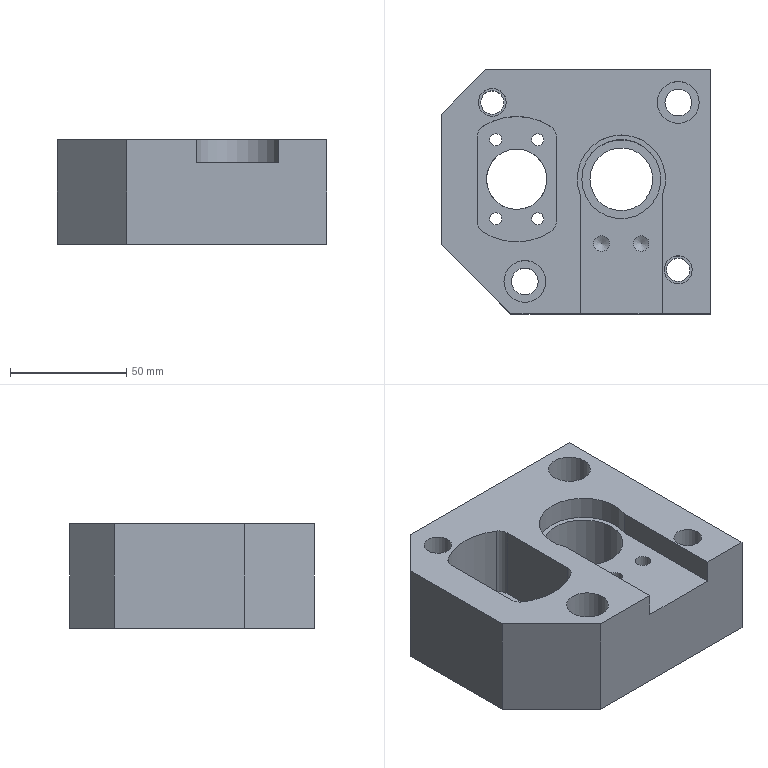Part | NX | features 26 2 | 1 solid | 45 faces | box 116 x 105 x 45 mm | volume 375782 mm3 | cylinder 24 | plane 19 | cone 2 | commonest cylinder face diameters 5.2 x4 10 x4 6.8 x2 10.001 x2 11.5 x2 12 x2
STEP:
#1=CARTESIAN_POINT('',(1753.,-18.439,-68.));
#2=VERTEX_POINT('',#1);
#3=CARTESIAN_POINT('',(1753.,18.439,-68.));
#4=VERTEX_POINT('',#3);
#5=CARTESIAN_POINT('',(1753.,211.,-68.));
#6=DIRECTION('',(0.,1.,0.));
#7=VECTOR('',#6,1000.);
#8=LINE('',#5,#7);
#9=EDGE_CURVE('',#2,#4,#8,.T.);
#10=ORIENTED_EDGE('',*,*,#9,.F.);
#11=CARTESIAN_POINT('',(1750.727,-22.63,-68.));
#12=VERTEX_POINT('',#11);
#13=CARTESIAN_POINT('',(1748.,-18.439,-68.));
#14=DIRECTION('',(0.,0.,1.));
#15=DIRECTION('',(-1.,0.,0.));
#16=AXIS2_PLACEMENT_3D('',#13,#14,#15);
#17=CIRCLE('',#16,5.);
#18=EDGE_CURVE('',#12,#2,#17,.T.);
#19=ORIENTED_EDGE('',*,*,#18,.F.);
#20=CARTESIAN_POINT('',(1721.273,-22.63,-68.));
#21=VERTEX_POINT('',#20);
#22=CARTESIAN_POINT('',(1736.,0.,-68.));
#23=DIRECTION('',(0.,0.,1.));
#24=DIRECTION('',(-1.,0.,0.));
#25=AXIS2_PLACEMENT_3D('',#22,#23,#24);
#26=CIRCLE('',#25,27.);
#27=EDGE_CURVE('',#21,#12,#26,.T.);
#28=ORIENTED_EDGE('',*,*,#27,.F.);
#29=CARTESIAN_POINT('',(1719.,-18.439,-68.));
#30=VERTEX_POINT('',#29);
#31=CARTESIAN_POINT('',(1724.,-18.439,-68.));
#32=DIRECTION('',(0.,0.,1.));
#33=DIRECTION('',(-1.,0.,0.));
#34=AXIS2_PLACEMENT_3D('',#31,#32,#33);
#35=CIRCLE('',#34,5.);
#36=EDGE_CURVE('',#30,#21,#35,.T.);
#37=ORIENTED_EDGE('',*,*,#36,.F.);
#38=CARTESIAN_POINT('',(1719.,18.439,-68.));
#39=VERTEX_POINT('',#38);
#40=CARTESIAN_POINT('',(1719.,211.,-68.));
#41=DIRECTION('',(0.,-1.,0.));
#42=VECTOR('',#41,1000.);
#43=LINE('',#40,#42);
#44=EDGE_CURVE('',#39,#30,#43,.T.);
#45=ORIENTED_EDGE('',*,*,#44,.F.);
#46=CARTESIAN_POINT('',(1721.273,22.63,-68.));
#47=VERTEX_POINT('',#46);
#48=CARTESIAN_POINT('',(1724.,18.439,-68.));
#49=DIRECTION('',(0.,0.,1.));
#50=DIRECTION('',(-1.,0.,0.));
#51=AXIS2_PLACEMENT_3D('',#48,#49,#50);
#52=CIRCLE('',#51,5.);
#53=EDGE_CURVE('',#47,#39,#52,.T.);
#54=ORIENTED_EDGE('',*,*,#53,.F.);
#55=CARTESIAN_POINT('',(1750.727,22.63,-68.));
#56=VERTEX_POINT('',#55);
#57=CARTESIAN_POINT('',(1736.,0.,-68.));
#58=DIRECTION('',(0.,0.,1.));
#59=DIRECTION('',(-1.,0.,0.));
#60=AXIS2_PLACEMENT_3D('',#57,#58,#59);
#61=CIRCLE('',#60,27.);
#62=EDGE_CURVE('',#56,#47,#61,.T.);
#63=ORIENTED_EDGE('',*,*,#62,.F.);
#64=CARTESIAN_POINT('',(1748.,18.439,-68.));
#65=DIRECTION('',(0.,0.,1.));
#66=DIRECTION('',(-1.,0.,0.));
#67=AXIS2_PLACEMENT_3D('',#64,#65,#66);
#68=CIRCLE('',#67,5.);
#69=EDGE_CURVE('',#4,#56,#68,.T.);
#70=ORIENTED_EDGE('',*,*,#69,.F.);
#71=EDGE_LOOP('',(#10,#19,#28,#37,#45,#54,#63,#70));
#72=FACE_BOUND('',#71,.T.);
#73=CARTESIAN_POINT('',(1730.5,-44.,-68.));
#74=VERTEX_POINT('',#73);
#75=CARTESIAN_POINT('',(1739.5,-44.,-68.));
#76=DIRECTION('',(0.,0.,1.));
#77=DIRECTION('',(-1.,0.,0.));
#78=AXIS2_PLACEMENT_3D('',#75,#76,#77);
#79=CIRCLE('',#78,9.);
#80=EDGE_CURVE('',#74,#74,#79,.T.);
#81=ORIENTED_EDGE('',*,*,#80,.F.);
#82=EDGE_LOOP('',(#81));
#83=FACE_BOUND('',#82,.T.);
#84=CARTESIAN_POINT('',(1796.5,33.,-68.));
#85=VERTEX_POINT('',#84);
#86=CARTESIAN_POINT('',(1805.5,33.,-68.));
#87=DIRECTION('',(0.,0.,1.));
#88=DIRECTION('',(-1.,0.,0.));
#89=AXIS2_PLACEMENT_3D('',#86,#87,#88);
#90=CIRCLE('',#89,9.);
#91=EDGE_CURVE('',#85,#85,#90,.T.);
#92=ORIENTED_EDGE('',*,*,#91,.F.);
#93=EDGE_LOOP('',(#92));
#94=FACE_BOUND('',#93,.T.);
#95=CARTESIAN_POINT('',(1719.5,33.,-68.));
#96=VERTEX_POINT('',#95);
#97=CARTESIAN_POINT('',(1725.5,33.,-68.));
#98=DIRECTION('',(0.,0.,-1.));
#99=DIRECTION('',(-1.,0.,0.));
#100=AXIS2_PLACEMENT_3D('',#97,#98,#99);
#101=CIRCLE('',#100,6.);
#102=EDGE_CURVE('',#96,#96,#101,.T.);
#103=ORIENTED_EDGE('',*,*,#102,.T.);
#104=EDGE_LOOP('',(#103));
#105=FACE_BOUND('',#104,.T.);
#106=CARTESIAN_POINT('',(1799.5,-39.,-68.));
#107=VERTEX_POINT('',#106);
#108=CARTESIAN_POINT('',(1805.5,-39.,-68.));
#109=DIRECTION('',(0.,0.,-1.));
#110=DIRECTION('',(-1.,0.,0.));
#111=AXIS2_PLACEMENT_3D('',#108,#109,#110);
#112=CIRCLE('',#111,6.);
#113=EDGE_CURVE('',#107,#107,#112,.T.);
#114=ORIENTED_EDGE('',*,*,#113,.T.);
#115=EDGE_LOOP('',(#114));
#116=FACE_BOUND('',#115,.T.);
#117=CARTESIAN_POINT('',(1722.5,47.,-68.));
#118=VERTEX_POINT('',#117);
#119=CARTESIAN_POINT('',(1703.5,28.,-68.));
#120=VERTEX_POINT('',#119);
#121=CARTESIAN_POINT('',(1249.,-426.5,-68.));
#122=DIRECTION('',(-0.7071,-0.7071,0.));
#123=VECTOR('',#122,1000.);
#124=LINE('',#121,#123);
#125=EDGE_CURVE('',#118,#120,#124,.T.);
#126=ORIENTED_EDGE('',*,*,#125,.T.);
#127=CARTESIAN_POINT('',(1703.5,-28.,-68.));
#128=VERTEX_POINT('',#127);
#129=CARTESIAN_POINT('',(1703.5,0.,-68.));
#130=DIRECTION('',(0.,-1.,0.));
#131=VECTOR('',#130,1000.);
#132=LINE('',#129,#131);
#133=EDGE_CURVE('',#120,#128,#132,.T.);
#134=ORIENTED_EDGE('',*,*,#133,.T.);
#135=CARTESIAN_POINT('',(1733.5,-58.,-68.));
#136=VERTEX_POINT('',#135);
#137=CARTESIAN_POINT('',(1733.5,-58.,-68.));
#138=DIRECTION('',(0.7071,-0.7071,0.));
#139=VECTOR('',#138,1000.);
#140=LINE('',#137,#139);
#141=EDGE_CURVE('',#128,#136,#140,.T.);
#142=ORIENTED_EDGE('',*,*,#141,.T.);
#143=CARTESIAN_POINT('',(1763.4,-58.,-68.));
#144=VERTEX_POINT('',#143);
#145=CARTESIAN_POINT('',(1781.,-58.,-68.));
#146=DIRECTION('',(1.,0.,0.));
#147=VECTOR('',#146,1000.);
#148=LINE('',#145,#147);
#149=EDGE_CURVE('',#136,#144,#148,.T.);
#150=ORIENTED_EDGE('',*,*,#149,.T.);
#151=CARTESIAN_POINT('',(1763.4,-7.158,-68.));
#152=VERTEX_POINT('',#151);
#153=CARTESIAN_POINT('',(1763.4,206.,-68.));
#154=DIRECTION('',(0.,-1.,0.));
#155=VECTOR('',#154,1000.);
#156=LINE('',#153,#155);
#157=EDGE_CURVE('',#152,#144,#156,.T.);
#158=ORIENTED_EDGE('',*,*,#157,.F.);
#159=CARTESIAN_POINT('',(1798.6,-7.158,-68.));
#160=VERTEX_POINT('',#159);
#161=CARTESIAN_POINT('',(1781.,0.,-68.));
#162=DIRECTION('',(0.,0.,1.));
#163=DIRECTION('',(1.,0.,0.));
#164=AXIS2_PLACEMENT_3D('',#161,#162,#163);
#165=CIRCLE('',#164,19.);
#166=EDGE_CURVE('',#160,#152,#165,.T.);
#167=ORIENTED_EDGE('',*,*,#166,.F.);
#168=CARTESIAN_POINT('',(1798.6,-58.,-68.));
#169=VERTEX_POINT('',#168);
#170=CARTESIAN_POINT('',(1798.6,206.,-68.));
#171=DIRECTION('',(0.,1.,0.));
#172=VECTOR('',#171,1000.);
#173=LINE('',#170,#172);
#174=EDGE_CURVE('',#169,#160,#173,.T.);
#175=ORIENTED_EDGE('',*,*,#174,.F.);
#176=CARTESIAN_POINT('',(1819.5,-58.,-68.));
#177=VERTEX_POINT('',#176);
#178=CARTESIAN_POINT('',(1781.,-58.,-68.));
#179=DIRECTION('',(1.,0.,0.));
#180=VECTOR('',#179,1000.);
#181=LINE('',#178,#180);
#182=EDGE_CURVE('',#169,#177,#181,.T.);
#183=ORIENTED_EDGE('',*,*,#182,.T.);
#184=CARTESIAN_POINT('',(1819.5,47.,-68.));
#185=VERTEX_POINT('',#184);
#186=CARTESIAN_POINT('',(1819.5,0.,-68.));
#187=DIRECTION('',(0.,1.,0.));
#188=VECTOR('',#187,1000.);
#189=LINE('',#186,#188);
#190=EDGE_CURVE('',#177,#185,#189,.T.);
#191=ORIENTED_EDGE('',*,*,#190,.T.);
#192=CARTESIAN_POINT('',(1781.,47.,-68.));
#193=DIRECTION('',(-1.,0.,0.));
#194=VECTOR('',#193,1000.);
#195=LINE('',#192,#194);
#196=EDGE_CURVE('',#185,#118,#195,.T.);
#197=ORIENTED_EDGE('',*,*,#196,.T.);
#198=EDGE_LOOP('',(#126,#134,#142,#150,#158,#167,#175,#183,#191,#197));
#199=FACE_BOUND('',#198,.T.);
#200=CARTESIAN_POINT('',(616.5,206.,-68.));
#201=DIRECTION('',(0.,0.,-1.));
#202=DIRECTION('',(-1.,0.,0.));
#203=AXIS2_PLACEMENT_3D('',#200,#201,#202);
#204=PLANE('',#203);
#205=ADVANCED_FACE('',(#72,#83,#94,#105,#116,#199),#204,.F.);
#206=CARTESIAN_POINT('',(1722.5,47.,-113.));
#207=VERTEX_POINT('',#206);
#208=CARTESIAN_POINT('',(1819.5,47.,-113.));
#209=VERTEX_POINT('',#208);
#210=CARTESIAN_POINT('',(1781.,47.,-113.));
#211=DIRECTION('',(1.,0.,0.));
#212=VECTOR('',#211,1000.);
#213=LINE('',#210,#212);
#214=EDGE_CURVE('',#207,#209,#213,.T.);
#215=ORIENTED_EDGE('',*,*,#214,.F.);
#216=CARTESIAN_POINT('',(1722.5,47.,-123.5));
#217=DIRECTION('',(0.,0.,1.));
#218=VECTOR('',#217,1000.);
#219=LINE('',#216,#218);
#220=EDGE_CURVE('',#207,#118,#219,.T.);
#221=ORIENTED_EDGE('',*,*,#220,.T.);
#222=ORIENTED_EDGE('',*,*,#196,.F.);
#223=CARTESIAN_POINT('',(1819.5,47.,-123.5));
#224=DIRECTION('',(0.,0.,-1.));
#225=VECTOR('',#224,1000.);
#226=LINE('',#223,#225);
#227=EDGE_CURVE('',#185,#209,#226,.T.);
#228=ORIENTED_EDGE('',*,*,#227,.T.);
#229=EDGE_LOOP('',(#215,#221,#222,#228));
#230=FACE_BOUND('',#229,.T.);
#231=CARTESIAN_POINT('',(1781.,47.,-123.5));
#232=DIRECTION('',(0.,1.,0.));
#233=DIRECTION('',(0.,0.,1.));
#234=AXIS2_PLACEMENT_3D('',#231,#232,#233);
#235=PLANE('',#234);
#236=ADVANCED_FACE('',(#230),#235,.T.);
#237=ORIENTED_EDGE('',*,*,#133,.F.);
#238=CARTESIAN_POINT('',(1703.5,28.,-113.));
#239=VERTEX_POINT('',#238);
#240=CARTESIAN_POINT('',(1703.5,28.,-204.));
#241=DIRECTION('',(0.,0.,1.));
#242=VECTOR('',#241,1000.);
#243=LINE('',#240,#242);
#244=EDGE_CURVE('',#239,#120,#243,.T.);
#245=ORIENTED_EDGE('',*,*,#244,.F.);
#246=CARTESIAN_POINT('',(1703.5,-28.,-113.));
#247=VERTEX_POINT('',#246);
#248=CARTESIAN_POINT('',(1703.5,0.,-113.));
#249=DIRECTION('',(0.,1.,0.));
#250=VECTOR('',#249,1000.);
#251=LINE('',#248,#250);
#252=EDGE_CURVE('',#247,#239,#251,.T.);
#253=ORIENTED_EDGE('',*,*,#252,.F.);
#254=CARTESIAN_POINT('',(1703.5,-28.,-123.5));
#255=DIRECTION('',(0.,0.,1.));
#256=VECTOR('',#255,1000.);
#257=LINE('',#254,#256);
#258=EDGE_CURVE('',#247,#128,#257,.T.);
#259=ORIENTED_EDGE('',*,*,#258,.T.);
#260=EDGE_LOOP('',(#237,#245,#253,#259));
#261=FACE_BOUND('',#260,.T.);
#262=CARTESIAN_POINT('',(1703.5,0.,-123.5));
#263=DIRECTION('',(-1.,0.,0.));
#264=DIRECTION('',(0.,0.,1.));
#265=AXIS2_PLACEMENT_3D('',#262,#263,#264);
#266=PLANE('',#265);
#267=ADVANCED_FACE('',(#261),#266,.T.);
#268=CARTESIAN_POINT('',(1742.4,17.,-113.));
#269=VERTEX_POINT('',#268);
#270=CARTESIAN_POINT('',(1745.,17.,-113.));
#271=DIRECTION('',(0.,0.,-1.));
#272=DIRECTION('',(-1.,0.,0.));
#273=AXIS2_PLACEMENT_3D('',#270,#271,#272);
#274=CIRCLE('',#273,2.6);
#275=EDGE_CURVE('',#269,#269,#274,.T.);
#276=ORIENTED_EDGE('',*,*,#275,.F.);
#277=EDGE_LOOP('',(#276));
#278=FACE_BOUND('',#277,.T.);
#279=CARTESIAN_POINT('',(1742.4,-17.,-113.));
#280=VERTEX_POINT('',#279);
#281=CARTESIAN_POINT('',(1745.,-17.,-113.));
#282=DIRECTION('',(0.,0.,-1.));
#283=DIRECTION('',(-1.,0.,0.));
#284=AXIS2_PLACEMENT_3D('',#281,#282,#283);
#285=CIRCLE('',#284,2.6);
#286=EDGE_CURVE('',#280,#280,#285,.T.);
#287=ORIENTED_EDGE('',*,*,#286,.F.);
#288=EDGE_LOOP('',(#287));
#289=FACE_BOUND('',#288,.T.);
#290=CARTESIAN_POINT('',(1724.4,17.,-113.));
#291=VERTEX_POINT('',#290);
#292=CARTESIAN_POINT('',(1727.,17.,-113.));
#293=DIRECTION('',(0.,0.,-1.));
#294=DIRECTION('',(-1.,0.,0.));
#295=AXIS2_PLACEMENT_3D('',#292,#293,#294);
#296=CIRCLE('',#295,2.6);
#297=EDGE_CURVE('',#291,#291,#296,.T.);
#298=ORIENTED_EDGE('',*,*,#297,.F.);
#299=EDGE_LOOP('',(#298));
#300=FACE_BOUND('',#299,.T.);
#301=CARTESIAN_POINT('',(1724.4,-17.,-113.));
#302=VERTEX_POINT('',#301);
#303=CARTESIAN_POINT('',(1727.,-17.,-113.));
#304=DIRECTION('',(0.,0.,-1.));
#305=DIRECTION('',(-1.,0.,0.));
#306=AXIS2_PLACEMENT_3D('',#303,#304,#305);
#307=CIRCLE('',#306,2.6);
#308=EDGE_CURVE('',#302,#302,#307,.T.);
#309=ORIENTED_EDGE('',*,*,#308,.F.);
#310=EDGE_LOOP('',(#309));
#311=FACE_BOUND('',#310,.T.);
#312=CARTESIAN_POINT('',(1800.499,-39.,-113.));
#313=VERTEX_POINT('',#312);
#314=CARTESIAN_POINT('',(1805.5,-39.,-113.));
#315=DIRECTION('',(0.,0.,-1.));
#316=DIRECTION('',(-1.,0.,0.));
#317=AXIS2_PLACEMENT_3D('',#314,#315,#316);
#318=CIRCLE('',#317,5.);
#319=EDGE_CURVE('',#313,#313,#318,.T.);
#320=ORIENTED_EDGE('',*,*,#319,.F.);
#321=EDGE_LOOP('',(#320));
#322=FACE_BOUND('',#321,.T.);
#323=CARTESIAN_POINT('',(1799.75,33.,-113.));
#324=VERTEX_POINT('',#323);
#325=CARTESIAN_POINT('',(1805.5,33.,-113.));
#326=DIRECTION('',(0.,0.,-1.));
#327=DIRECTION('',(-1.,0.,0.));
#328=AXIS2_PLACEMENT_3D('',#325,#326,#327);
#329=CIRCLE('',#328,5.75);
#330=EDGE_CURVE('',#324,#324,#329,.T.);
#331=ORIENTED_EDGE('',*,*,#330,.F.);
#332=EDGE_LOOP('',(#331));
#333=FACE_BOUND('',#332,.T.);
#334=CARTESIAN_POINT('',(1794.5,0.,-113.));
#335=VERTEX_POINT('',#334);
#336=CARTESIAN_POINT('',(1781.,0.,-113.));
#337=DIRECTION('',(0.,0.,-1.));
#338=DIRECTION('',(1.,0.,0.));
#339=AXIS2_PLACEMENT_3D('',#336,#337,#338);
#340=CIRCLE('',#339,13.5);
#341=EDGE_CURVE('',#335,#335,#340,.T.);
#342=ORIENTED_EDGE('',*,*,#341,.F.);
#343=EDGE_LOOP('',(#342));
#344=FACE_BOUND('',#343,.T.);
#345=CARTESIAN_POINT('',(1733.75,-44.,-113.));
#346=VERTEX_POINT('',#345);
#347=CARTESIAN_POINT('',(1739.5,-44.,-113.));
#348=DIRECTION('',(0.,0.,-1.));
#349=DIRECTION('',(-1.,0.,0.));
#350=AXIS2_PLACEMENT_3D('',#347,#348,#349);
#351=CIRCLE('',#350,5.75);
#352=EDGE_CURVE('',#346,#346,#351,.T.);
#353=ORIENTED_EDGE('',*,*,#352,.F.);
#354=EDGE_LOOP('',(#353));
#355=FACE_BOUND('',#354,.T.);
#356=CARTESIAN_POINT('',(1720.499,33.,-113.));
#357=VERTEX_POINT('',#356);
#358=CARTESIAN_POINT('',(1725.5,33.,-113.));
#359=DIRECTION('',(0.,0.,-1.));
#360=DIRECTION('',(-1.,0.,0.));
#361=AXIS2_PLACEMENT_3D('',#358,#359,#360);
#362=CIRCLE('',#361,5.);
#363=EDGE_CURVE('',#357,#357,#362,.T.);
#364=ORIENTED_EDGE('',*,*,#363,.F.);
#365=EDGE_LOOP('',(#364));
#366=FACE_BOUND('',#365,.T.);
#367=CARTESIAN_POINT('',(1723.,0.,-113.));
#368=VERTEX_POINT('',#367);
#369=CARTESIAN_POINT('',(1736.,0.,-113.));
#370=DIRECTION('',(0.,0.,1.));
#371=DIRECTION('',(-1.,0.,0.));
#372=AXIS2_PLACEMENT_3D('',#369,#370,#371);
#373=CIRCLE('',#372,13.);
#374=EDGE_CURVE('',#368,#368,#373,.T.);
#375=ORIENTED_EDGE('',*,*,#374,.T.);
#376=EDGE_LOOP('',(#375));
#377=FACE_BOUND('',#376,.T.);
#378=ORIENTED_EDGE('',*,*,#252,.T.);
#379=CARTESIAN_POINT('',(1111.75,-563.75,-113.));
#380=DIRECTION('',(-0.7071,-0.7071,0.));
#381=VECTOR('',#380,1000.);
#382=LINE('',#379,#381);
#383=EDGE_CURVE('',#207,#239,#382,.T.);
#384=ORIENTED_EDGE('',*,*,#383,.F.);
#385=ORIENTED_EDGE('',*,*,#214,.T.);
#386=CARTESIAN_POINT('',(1819.5,-58.,-113.));
#387=VERTEX_POINT('',#386);
#388=CARTESIAN_POINT('',(1819.5,0.,-113.));
#389=DIRECTION('',(0.,-1.,0.));
#390=VECTOR('',#389,1000.);
#391=LINE('',#388,#390);
#392=EDGE_CURVE('',#209,#387,#391,.T.);
#393=ORIENTED_EDGE('',*,*,#392,.T.);
#394=CARTESIAN_POINT('',(1733.5,-58.,-113.));
#395=VERTEX_POINT('',#394);
#396=CARTESIAN_POINT('',(1781.,-58.,-113.));
#397=DIRECTION('',(-1.,0.,0.));
#398=VECTOR('',#397,1000.);
#399=LINE('',#396,#398);
#400=EDGE_CURVE('',#387,#395,#399,.T.);
#401=ORIENTED_EDGE('',*,*,#400,.T.);
#402=CARTESIAN_POINT('',(1114.75,560.75,-113.));
#403=DIRECTION('',(-0.7071,0.7071,0.));
#404=VECTOR('',#403,1000.);
#405=LINE('',#402,#404);
#406=EDGE_CURVE('',#395,#247,#405,.T.);
#407=ORIENTED_EDGE('',*,*,#406,.T.);
#408=EDGE_LOOP('',(#378,#384,#385,#393,#401,#407));
#409=FACE_BOUND('',#408,.T.);
#410=CARTESIAN_POINT('',(551.,-3.,-113.));
#411=DIRECTION('',(0.,0.,-1.));
#412=DIRECTION('',(1.,0.,0.));
#413=AXIS2_PLACEMENT_3D('',#410,#411,#412);
#414=PLANE('',#413);
#415=ADVANCED_FACE('',(#278,#289,#300,#311,#322,#333,#344,#355,#366,#377,#409),#414,.T.);
#416=CARTESIAN_POINT('',(1764.,0.,-108.));
#417=VERTEX_POINT('',#416);
#418=CARTESIAN_POINT('',(1781.,0.,-108.));
#419=DIRECTION('',(0.,0.,1.));
#420=DIRECTION('',(-1.,0.,0.));
#421=AXIS2_PLACEMENT_3D('',#418,#419,#420);
#422=CIRCLE('',#421,17.);
#423=EDGE_CURVE('',#417,#417,#422,.T.);
#424=ORIENTED_EDGE('',*,*,#423,.F.);
#425=EDGE_LOOP('',(#424));
#426=FACE_BOUND('',#425,.T.);
#427=CARTESIAN_POINT('',(1764.,0.,-78.));
#428=VERTEX_POINT('',#427);
#429=CARTESIAN_POINT('',(1781.,0.,-78.));
#430=DIRECTION('',(0.,0.,-1.));
#431=DIRECTION('',(-1.,0.,0.));
#432=AXIS2_PLACEMENT_3D('',#429,#430,#431);
#433=CIRCLE('',#432,17.);
#434=EDGE_CURVE('',#428,#428,#433,.T.);
#435=ORIENTED_EDGE('',*,*,#434,.F.);
#436=EDGE_LOOP('',(#435));
#437=FACE_BOUND('',#436,.T.);
#438=CARTESIAN_POINT('',(1781.,0.,512.));
#439=DIRECTION('',(0.,0.,-1.));
#440=DIRECTION('',(-1.,0.,0.));
#441=AXIS2_PLACEMENT_3D('',#438,#439,#440);
#442=CYLINDRICAL_SURFACE('',#441,17.);
#443=ADVANCED_FACE('',(#426,#437),#442,.F.);
#444=CARTESIAN_POINT('',(1819.5,-58.,-123.5));
#445=DIRECTION('',(0.,0.,-1.));
#446=VECTOR('',#445,1000.);
#447=LINE('',#444,#446);
#448=EDGE_CURVE('',#177,#387,#447,.T.);
#449=ORIENTED_EDGE('',*,*,#448,.T.);
#450=ORIENTED_EDGE('',*,*,#392,.F.);
#451=ORIENTED_EDGE('',*,*,#227,.F.);
#452=ORIENTED_EDGE('',*,*,#190,.F.);
#453=EDGE_LOOP('',(#449,#450,#451,#452));
#454=FACE_BOUND('',#453,.T.);
#455=CARTESIAN_POINT('',(1819.5,0.,-123.5));
#456=DIRECTION('',(1.,0.,0.));
#457=DIRECTION('',(0.,0.,-1.));
#458=AXIS2_PLACEMENT_3D('',#455,#456,#457);
#459=PLANE('',#458);
#460=ADVANCED_FACE('',(#454),#459,.T.);
#461=ORIENTED_EDGE('',*,*,#149,.F.);
#462=CARTESIAN_POINT('',(1733.5,-58.,-123.5));
#463=DIRECTION('',(0.,0.,-1.));
#464=VECTOR('',#463,1000.);
#465=LINE('',#462,#464);
#466=EDGE_CURVE('',#136,#395,#465,.T.);
#467=ORIENTED_EDGE('',*,*,#466,.T.);
#468=ORIENTED_EDGE('',*,*,#400,.F.);
#469=ORIENTED_EDGE('',*,*,#448,.F.);
#470=ORIENTED_EDGE('',*,*,#182,.F.);
#471=CARTESIAN_POINT('',(1798.6,-58.,-78.));
#472=VERTEX_POINT('',#471);
#473=CARTESIAN_POINT('',(1798.6,-58.,-58.));
#474=DIRECTION('',(0.,0.,1.));
#475=VECTOR('',#474,1000.);
#476=LINE('',#473,#475);
#477=EDGE_CURVE('',#472,#169,#476,.T.);
#478=ORIENTED_EDGE('',*,*,#477,.F.);
#479=CARTESIAN_POINT('',(1763.4,-58.,-78.));
#480=VERTEX_POINT('',#479);
#481=CARTESIAN_POINT('',(1781.,-58.,-78.));
#482=DIRECTION('',(-1.,0.,0.));
#483=VECTOR('',#482,1000.);
#484=LINE('',#481,#483);
#485=EDGE_CURVE('',#472,#480,#484,.T.);
#486=ORIENTED_EDGE('',*,*,#485,.T.);
#487=CARTESIAN_POINT('',(1763.4,-58.,-123.5));
#488=DIRECTION('',(0.,0.,1.));
#489=VECTOR('',#488,1000.);
#490=LINE('',#487,#489);
#491=EDGE_CURVE('',#480,#144,#490,.T.);
#492=ORIENTED_EDGE('',*,*,#491,.T.);
#493=EDGE_LOOP('',(#461,#467,#468,#469,#470,#478,#486,#492));
#494=FACE_BOUND('',#493,.T.);
#495=CARTESIAN_POINT('',(1781.,-58.,-123.5));
#496=DIRECTION('',(0.,-1.,0.));
#497=DIRECTION('',(0.,0.,-1.));
#498=AXIS2_PLACEMENT_3D('',#495,#496,#497);
#499=PLANE('',#498);
#500=ADVANCED_FACE('',(#494),#499,.T.);
#501=CARTESIAN_POINT('',(1800.499,-39.,-88.5));
#502=VERTEX_POINT('',#501);
#503=CARTESIAN_POINT('',(1805.5,-39.,-88.5));
#504=DIRECTION('',(0.,0.,1.));
#505=DIRECTION('',(-1.,0.,0.));
#506=AXIS2_PLACEMENT_3D('',#503,#504,#505);
#507=CIRCLE('',#506,5.);
#508=EDGE_CURVE('',#502,#502,#507,.T.);
#509=ORIENTED_EDGE('',*,*,#508,.T.);
#510=EDGE_LOOP('',(#509));
#511=FACE_BOUND('',#510,.T.);
#512=ORIENTED_EDGE('',*,*,#319,.T.);
#513=EDGE_LOOP('',(#512));
#514=FACE_BOUND('',#513,.T.);
#515=CARTESIAN_POINT('',(1805.5,-39.,541.5));
#516=DIRECTION('',(0.,0.,-1.));
#517=DIRECTION('',(-1.,0.,0.));
#518=AXIS2_PLACEMENT_3D('',#515,#516,#517);
#519=CYLINDRICAL_SURFACE('',#518,5.);
#520=ADVANCED_FACE('',(#511,#514),#519,.F.);
#521=CARTESIAN_POINT('',(1720.499,33.,-88.5));
#522=VERTEX_POINT('',#521);
#523=CARTESIAN_POINT('',(1725.5,33.,-88.5));
#524=DIRECTION('',(0.,0.,1.));
#525=DIRECTION('',(-1.,0.,0.));
#526=AXIS2_PLACEMENT_3D('',#523,#524,#525);
#527=CIRCLE('',#526,5.);
#528=EDGE_CURVE('',#522,#522,#527,.T.);
#529=ORIENTED_EDGE('',*,*,#528,.T.);
#530=EDGE_LOOP('',(#529));
#531=FACE_BOUND('',#530,.T.);
#532=ORIENTED_EDGE('',*,*,#363,.T.);
#533=EDGE_LOOP('',(#532));
#534=FACE_BOUND('',#533,.T.);
#535=CARTESIAN_POINT('',(1725.5,33.,541.5));
#536=DIRECTION('',(0.,0.,-1.));
#537=DIRECTION('',(-1.,0.,0.));
#538=AXIS2_PLACEMENT_3D('',#535,#536,#537);
#539=CYLINDRICAL_SURFACE('',#538,5.);
#540=ADVANCED_FACE('',(#531,#534),#539,.F.);
#541=CARTESIAN_POINT('',(1799.75,33.,-88.5));
#542=VERTEX_POINT('',#541);
#543=CARTESIAN_POINT('',(1805.5,33.,-88.5));
#544=DIRECTION('',(0.,0.,1.));
#545=DIRECTION('',(-1.,0.,0.));
#546=AXIS2_PLACEMENT_3D('',#543,#544,#545);
#547=CIRCLE('',#546,5.75);
#548=EDGE_CURVE('',#542,#542,#547,.T.);
#549=ORIENTED_EDGE('',*,*,#548,.T.);
#550=EDGE_LOOP('',(#549));
#551=FACE_BOUND('',#550,.T.);
#552=ORIENTED_EDGE('',*,*,#330,.T.);
#553=EDGE_LOOP('',(#552));
#554=FACE_BOUND('',#553,.T.);
#555=CARTESIAN_POINT('',(1805.5,33.,-66.5));
#556=DIRECTION('',(0.,0.,-1.));
#557=DIRECTION('',(1.,0.,0.));
#558=AXIS2_PLACEMENT_3D('',#555,#556,#557);
#559=CYLINDRICAL_SURFACE('',#558,5.75);
#560=ADVANCED_FACE('',(#551,#554),#559,.F.);
#561=CARTESIAN_POINT('',(1733.75,-44.,-88.5));
#562=VERTEX_POINT('',#561);
#563=CARTESIAN_POINT('',(1739.5,-44.,-88.5));
#564=DIRECTION('',(0.,0.,1.));
#565=DIRECTION('',(-1.,0.,0.));
#566=AXIS2_PLACEMENT_3D('',#563,#564,#565);
#567=CIRCLE('',#566,5.75);
#568=EDGE_CURVE('',#562,#562,#567,.T.);
#569=ORIENTED_EDGE('',*,*,#568,.T.);
#570=EDGE_LOOP('',(#569));
#571=FACE_BOUND('',#570,.T.);
#572=ORIENTED_EDGE('',*,*,#352,.T.);
#573=EDGE_LOOP('',(#572));
#574=FACE_BOUND('',#573,.T.);
#575=CARTESIAN_POINT('',(1739.5,-44.,-66.5));
#576=DIRECTION('',(0.,0.,-1.));
#577=DIRECTION('',(1.,0.,0.));
#578=AXIS2_PLACEMENT_3D('',#575,#576,#577);
#579=CYLINDRICAL_SURFACE('',#578,5.75);
#580=ADVANCED_FACE('',(#571,#574),#579,.F.);
#581=CARTESIAN_POINT('',(1767.5,0.,-108.));
#582=VERTEX_POINT('',#581);
#583=CARTESIAN_POINT('',(1781.,0.,-108.));
#584=DIRECTION('',(0.,0.,1.));
#585=DIRECTION('',(-1.,0.,0.));
#586=AXIS2_PLACEMENT_3D('',#583,#584,#585);
#587=CIRCLE('',#586,13.5);
#588=EDGE_CURVE('',#582,#582,#587,.T.);
#589=ORIENTED_EDGE('',*,*,#588,.T.);
#590=EDGE_LOOP('',(#589));
#591=FACE_BOUND('',#590,.T.);
#592=ORIENTED_EDGE('',*,*,#341,.T.);
#593=EDGE_LOOP('',(#592));
#594=FACE_BOUND('',#593,.T.);
#595=CARTESIAN_POINT('',(1781.,0.,542.));
#596=DIRECTION('',(0.,0.,-1.));
#597=DIRECTION('',(-1.,0.,0.));
#598=AXIS2_PLACEMENT_3D('',#595,#596,#597);
#599=CYLINDRICAL_SURFACE('',#598,13.5);
#600=ADVANCED_FACE('',(#591,#594),#599,.F.);
#601=CARTESIAN_POINT('',(1731.5,33.,-88.5));
#602=VERTEX_POINT('',#601);
#603=CARTESIAN_POINT('',(1725.5,33.,-88.5));
#604=DIRECTION('',(0.,0.,-1.));
#605=DIRECTION('',(1.,0.,0.));
#606=AXIS2_PLACEMENT_3D('',#603,#604,#605);
#607=CIRCLE('',#606,6.);
#608=EDGE_CURVE('',#602,#602,#607,.T.);
#609=ORIENTED_EDGE('',*,*,#608,.T.);
#610=EDGE_LOOP('',(#609));
#611=FACE_BOUND('',#610,.T.);
#612=ORIENTED_EDGE('',*,*,#102,.F.);
#613=EDGE_LOOP('',(#612));
#614=FACE_BOUND('',#613,.T.);
#615=CARTESIAN_POINT('',(1725.5,33.,541.5));
#616=DIRECTION('',(0.,0.,-1.));
#617=DIRECTION('',(-1.,0.,0.));
#618=AXIS2_PLACEMENT_3D('',#615,#616,#617);
#619=CYLINDRICAL_SURFACE('',#618,6.);
#620=ADVANCED_FACE('',(#611,#614),#619,.F.);
#621=ORIENTED_EDGE('',*,*,#113,.F.);
#622=EDGE_LOOP('',(#621));
#623=FACE_BOUND('',#622,.T.);
#624=CARTESIAN_POINT('',(1811.5,-39.,-88.5));
#625=VERTEX_POINT('',#624);
#626=CARTESIAN_POINT('',(1805.5,-39.,-88.5));
#627=DIRECTION('',(0.,0.,-1.));
#628=DIRECTION('',(1.,0.,0.));
#629=AXIS2_PLACEMENT_3D('',#626,#627,#628);
#630=CIRCLE('',#629,6.);
#631=EDGE_CURVE('',#625,#625,#630,.T.);
#632=ORIENTED_EDGE('',*,*,#631,.T.);
#633=EDGE_LOOP('',(#632));
#634=FACE_BOUND('',#633,.T.);
#635=CARTESIAN_POINT('',(1805.5,-39.,541.5));
#636=DIRECTION('',(0.,0.,-1.));
#637=DIRECTION('',(-1.,0.,0.));
#638=AXIS2_PLACEMENT_3D('',#635,#636,#637);
#639=CYLINDRICAL_SURFACE('',#638,6.);
#640=ADVANCED_FACE('',(#623,#634),#639,.F.);
#641=CARTESIAN_POINT('',(1796.5,33.,-88.5));
#642=VERTEX_POINT('',#641);
#643=CARTESIAN_POINT('',(1805.5,33.,-88.5));
#644=DIRECTION('',(0.,0.,1.));
#645=DIRECTION('',(-1.,0.,0.));
#646=AXIS2_PLACEMENT_3D('',#643,#644,#645);
#647=CIRCLE('',#646,9.);
#648=EDGE_CURVE('',#642,#642,#647,.T.);
#649=ORIENTED_EDGE('',*,*,#648,.F.);
#650=EDGE_LOOP('',(#649));
#651=FACE_BOUND('',#650,.T.);
#652=ORIENTED_EDGE('',*,*,#91,.T.);
#653=EDGE_LOOP('',(#652));
#654=FACE_BOUND('',#653,.T.);
#655=CARTESIAN_POINT('',(1805.5,33.,-68.5));
#656=DIRECTION('',(0.,0.,-1.));
#657=DIRECTION('',(1.,0.,0.));
#658=AXIS2_PLACEMENT_3D('',#655,#656,#657);
#659=CYLINDRICAL_SURFACE('',#658,9.);
#660=ADVANCED_FACE('',(#651,#654),#659,.F.);
#661=CARTESIAN_POINT('',(1730.5,-44.,-88.5));
#662=VERTEX_POINT('',#661);
#663=CARTESIAN_POINT('',(1739.5,-44.,-88.5));
#664=DIRECTION('',(0.,0.,1.));
#665=DIRECTION('',(-1.,0.,0.));
#666=AXIS2_PLACEMENT_3D('',#663,#664,#665);
#667=CIRCLE('',#666,9.);
#668=EDGE_CURVE('',#662,#662,#667,.T.);
#669=ORIENTED_EDGE('',*,*,#668,.F.);
#670=EDGE_LOOP('',(#669));
#671=FACE_BOUND('',#670,.T.);
#672=ORIENTED_EDGE('',*,*,#80,.T.);
#673=EDGE_LOOP('',(#672));
#674=FACE_BOUND('',#673,.T.);
#675=CARTESIAN_POINT('',(1739.5,-44.,-68.5));
#676=DIRECTION('',(0.,0.,-1.));
#677=DIRECTION('',(1.,0.,0.));
#678=AXIS2_PLACEMENT_3D('',#675,#676,#677);
#679=CYLINDRICAL_SURFACE('',#678,9.);
#680=ADVANCED_FACE('',(#671,#674),#679,.F.);
#681=ORIENTED_EDGE('',*,*,#668,.T.);
#682=EDGE_LOOP('',(#681));
#683=FACE_BOUND('',#682,.T.);
#684=ORIENTED_EDGE('',*,*,#568,.F.);
#685=EDGE_LOOP('',(#684));
#686=FACE_BOUND('',#685,.T.);
#687=CARTESIAN_POINT('',(1796.5,-2.,-88.5));
#688=DIRECTION('',(0.,0.,-1.));
#689=DIRECTION('',(-1.,0.,0.));
#690=AXIS2_PLACEMENT_3D('',#687,#688,#689);
#691=PLANE('',#690);
#692=ADVANCED_FACE('',(#683,#686),#691,.F.);
#693=ORIENTED_EDGE('',*,*,#608,.F.);
#694=EDGE_LOOP('',(#693));
#695=FACE_BOUND('',#694,.T.);
#696=ORIENTED_EDGE('',*,*,#528,.F.);
#697=EDGE_LOOP('',(#696));
#698=FACE_BOUND('',#697,.T.);
#699=CARTESIAN_POINT('',(1782.5,33.,-88.5));
#700=DIRECTION('',(0.,0.,-1.));
#701=DIRECTION('',(-1.,0.,0.));
#702=AXIS2_PLACEMENT_3D('',#699,#700,#701);
#703=PLANE('',#702);
#704=ADVANCED_FACE('',(#695,#698),#703,.F.);
#705=ORIENTED_EDGE('',*,*,#631,.F.);
#706=EDGE_LOOP('',(#705));
#707=FACE_BOUND('',#706,.T.);
#708=ORIENTED_EDGE('',*,*,#508,.F.);
#709=EDGE_LOOP('',(#708));
#710=FACE_BOUND('',#709,.T.);
#711=CARTESIAN_POINT('',(1805.5,3.,-88.5));
#712=DIRECTION('',(0.,0.,-1.));
#713=DIRECTION('',(-1.,0.,0.));
#714=AXIS2_PLACEMENT_3D('',#711,#712,#713);
#715=PLANE('',#714);
#716=ADVANCED_FACE('',(#707,#710),#715,.F.);
#717=ORIENTED_EDGE('',*,*,#423,.T.);
#718=EDGE_LOOP('',(#717));
#719=FACE_BOUND('',#718,.T.);
#720=ORIENTED_EDGE('',*,*,#588,.F.);
#721=EDGE_LOOP('',(#720));
#722=FACE_BOUND('',#721,.T.);
#723=CARTESIAN_POINT('',(1781.,0.,-108.));
#724=DIRECTION('',(0.,0.,1.));
#725=DIRECTION('',(1.,0.,0.));
#726=AXIS2_PLACEMENT_3D('',#723,#724,#725);
#727=PLANE('',#726);
#728=ADVANCED_FACE('',(#719,#722),#727,.T.);
#729=ORIENTED_EDGE('',*,*,#648,.T.);
#730=EDGE_LOOP('',(#729));
#731=FACE_BOUND('',#730,.T.);
#732=ORIENTED_EDGE('',*,*,#548,.F.);
#733=EDGE_LOOP('',(#732));
#734=FACE_BOUND('',#733,.T.);
#735=CARTESIAN_POINT('',(1805.5,33.,-88.5));
#736=DIRECTION('',(0.,0.,-1.));
#737=DIRECTION('',(-1.,0.,0.));
#738=AXIS2_PLACEMENT_3D('',#735,#736,#737);
#739=PLANE('',#738);
#740=ADVANCED_FACE('',(#731,#734),#739,.F.);
#741=CARTESIAN_POINT('',(1736.,13.,-100.));
#742=VERTEX_POINT('',#741);
#743=CARTESIAN_POINT('',(1736.,0.,-100.));
#744=DIRECTION('',(0.,0.,-1.));
#745=DIRECTION('',(0.,1.,0.));
#746=AXIS2_PLACEMENT_3D('',#743,#744,#745);
#747=CIRCLE('',#746,13.);
#748=EDGE_CURVE('',#742,#742,#747,.T.);
#749=ORIENTED_EDGE('',*,*,#748,.F.);
#750=EDGE_LOOP('',(#749));
#751=FACE_BOUND('',#750,.T.);
#752=ORIENTED_EDGE('',*,*,#374,.F.);
#753=EDGE_LOOP('',(#752));
#754=FACE_BOUND('',#753,.T.);
#755=CARTESIAN_POINT('',(1736.,0.,-95.5));
#756=DIRECTION('',(0.,0.,1.));
#757=DIRECTION('',(1.,0.,0.));
#758=AXIS2_PLACEMENT_3D('',#755,#756,#757);
#759=CYLINDRICAL_SURFACE('',#758,13.);
#760=ADVANCED_FACE('',(#751,#754),#759,.F.);
#761=ORIENTED_EDGE('',*,*,#27,.T.);
#762=CARTESIAN_POINT('',(1750.727,-22.63,-100.));
#763=VERTEX_POINT('',#762);
#764=CARTESIAN_POINT('',(1750.727,-22.63,-95.5));
#765=DIRECTION('',(0.,0.,1.));
#766=VECTOR('',#765,1000.);
#767=LINE('',#764,#766);
#768=EDGE_CURVE('',#763,#12,#767,.T.);
#769=ORIENTED_EDGE('',*,*,#768,.F.);
#770=CARTESIAN_POINT('',(1721.273,-22.63,-100.));
#771=VERTEX_POINT('',#770);
#772=CARTESIAN_POINT('',(1736.,0.,-100.));
#773=DIRECTION('',(0.,0.,-1.));
#774=DIRECTION('',(0.,1.,0.));
#775=AXIS2_PLACEMENT_3D('',#772,#773,#774);
#776=CIRCLE('',#775,27.);
#777=EDGE_CURVE('',#763,#771,#776,.T.);
#778=ORIENTED_EDGE('',*,*,#777,.T.);
#779=CARTESIAN_POINT('',(1721.273,-22.63,-95.5));
#780=DIRECTION('',(0.,0.,-1.));
#781=VECTOR('',#780,1000.);
#782=LINE('',#779,#781);
#783=EDGE_CURVE('',#21,#771,#782,.T.);
#784=ORIENTED_EDGE('',*,*,#783,.F.);
#785=EDGE_LOOP('',(#761,#769,#778,#784));
#786=FACE_BOUND('',#785,.T.);
#787=CARTESIAN_POINT('',(1736.,0.,-95.5));
#788=DIRECTION('',(0.,0.,1.));
#789=DIRECTION('',(1.,0.,0.));
#790=AXIS2_PLACEMENT_3D('',#787,#788,#789);
#791=CYLINDRICAL_SURFACE('',#790,27.);
#792=ADVANCED_FACE('',(#786),#791,.F.);
#793=CARTESIAN_POINT('',(1719.,-18.439,-100.));
#794=VERTEX_POINT('',#793);
#795=CARTESIAN_POINT('',(1719.,18.439,-100.));
#796=VERTEX_POINT('',#795);
#797=CARTESIAN_POINT('',(1719.,0.,-100.));
#798=DIRECTION('',(0.,1.,0.));
#799=VECTOR('',#798,1000.);
#800=LINE('',#797,#799);
#801=EDGE_CURVE('',#794,#796,#800,.T.);
#802=ORIENTED_EDGE('',*,*,#801,.T.);
#803=CARTESIAN_POINT('',(1719.,18.439,-68.5));
#804=DIRECTION('',(0.,0.,-1.));
#805=VECTOR('',#804,1000.);
#806=LINE('',#803,#805);
#807=EDGE_CURVE('',#39,#796,#806,.T.);
#808=ORIENTED_EDGE('',*,*,#807,.F.);
#809=ORIENTED_EDGE('',*,*,#44,.T.);
#810=CARTESIAN_POINT('',(1719.,-18.439,-100.));
#811=DIRECTION('',(0.,0.,1.));
#812=VECTOR('',#811,1000.);
#813=LINE('',#810,#812);
#814=EDGE_CURVE('',#794,#30,#813,.T.);
#815=ORIENTED_EDGE('',*,*,#814,.F.);
#816=EDGE_LOOP('',(#802,#808,#809,#815));
#817=FACE_BOUND('',#816,.T.);
#818=CARTESIAN_POINT('',(1719.,0.,-95.5));
#819=DIRECTION('',(-1.,0.,0.));
#820=DIRECTION('',(0.,-1.,0.));
#821=AXIS2_PLACEMENT_3D('',#818,#819,#820);
#822=PLANE('',#821);
#823=ADVANCED_FACE('',(#817),#822,.F.);
#824=ORIENTED_EDGE('',*,*,#62,.T.);
#825=CARTESIAN_POINT('',(1721.273,22.63,-100.));
#826=VERTEX_POINT('',#825);
#827=CARTESIAN_POINT('',(1721.273,22.63,-95.5));
#828=DIRECTION('',(0.,0.,1.));
#829=VECTOR('',#828,1000.);
#830=LINE('',#827,#829);
#831=EDGE_CURVE('',#826,#47,#830,.T.);
#832=ORIENTED_EDGE('',*,*,#831,.F.);
#833=CARTESIAN_POINT('',(1750.727,22.63,-100.));
#834=VERTEX_POINT('',#833);
#835=CARTESIAN_POINT('',(1736.,0.,-100.));
#836=DIRECTION('',(0.,0.,-1.));
#837=DIRECTION('',(0.,1.,0.));
#838=AXIS2_PLACEMENT_3D('',#835,#836,#837);
#839=CIRCLE('',#838,27.);
#840=EDGE_CURVE('',#826,#834,#839,.T.);
#841=ORIENTED_EDGE('',*,*,#840,.T.);
#842=CARTESIAN_POINT('',(1750.727,22.63,-95.5));
#843=DIRECTION('',(0.,0.,-1.));
#844=VECTOR('',#843,1000.);
#845=LINE('',#842,#844);
#846=EDGE_CURVE('',#56,#834,#845,.T.);
#847=ORIENTED_EDGE('',*,*,#846,.F.);
#848=EDGE_LOOP('',(#824,#832,#841,#847));
#849=FACE_BOUND('',#848,.T.);
#850=CARTESIAN_POINT('',(1736.,0.,-95.5));
#851=DIRECTION('',(0.,0.,1.));
#852=DIRECTION('',(1.,0.,0.));
#853=AXIS2_PLACEMENT_3D('',#850,#851,#852);
#854=CYLINDRICAL_SURFACE('',#853,27.);
#855=ADVANCED_FACE('',(#849),#854,.F.);
#856=ORIENTED_EDGE('',*,*,#9,.T.);
#857=CARTESIAN_POINT('',(1753.,18.439,-100.));
#858=VERTEX_POINT('',#857);
#859=CARTESIAN_POINT('',(1753.,18.439,-100.));
#860=DIRECTION('',(0.,0.,1.));
#861=VECTOR('',#860,1000.);
#862=LINE('',#859,#861);
#863=EDGE_CURVE('',#858,#4,#862,.T.);
#864=ORIENTED_EDGE('',*,*,#863,.F.);
#865=CARTESIAN_POINT('',(1753.,-18.439,-100.));
#866=VERTEX_POINT('',#865);
#867=CARTESIAN_POINT('',(1753.,0.,-100.));
#868=DIRECTION('',(0.,-1.,0.));
#869=VECTOR('',#868,1000.);
#870=LINE('',#867,#869);
#871=EDGE_CURVE('',#858,#866,#870,.T.);
#872=ORIENTED_EDGE('',*,*,#871,.T.);
#873=CARTESIAN_POINT('',(1753.,-18.439,-68.5));
#874=DIRECTION('',(0.,0.,-1.));
#875=VECTOR('',#874,1000.);
#876=LINE('',#873,#875);
#877=EDGE_CURVE('',#2,#866,#876,.T.);
#878=ORIENTED_EDGE('',*,*,#877,.F.);
#879=EDGE_LOOP('',(#856,#864,#872,#878));
#880=FACE_BOUND('',#879,.T.);
#881=CARTESIAN_POINT('',(1753.,0.,-95.5));
#882=DIRECTION('',(1.,0.,0.));
#883=DIRECTION('',(0.,1.,0.));
#884=AXIS2_PLACEMENT_3D('',#881,#882,#883);
#885=PLANE('',#884);
#886=ADVANCED_FACE('',(#880),#885,.F.);
#887=CARTESIAN_POINT('',(1747.6,17.,-100.));
#888=VERTEX_POINT('',#887);
#889=CARTESIAN_POINT('',(1745.,17.,-100.));
#890=DIRECTION('',(0.,0.,-1.));
#891=DIRECTION('',(1.,0.,0.));
#892=AXIS2_PLACEMENT_3D('',#889,#890,#891);
#893=CIRCLE('',#892,2.6);
#894=EDGE_CURVE('',#888,#888,#893,.T.);
#895=ORIENTED_EDGE('',*,*,#894,.T.);
#896=EDGE_LOOP('',(#895));
#897=FACE_BOUND('',#896,.T.);
#898=CARTESIAN_POINT('',(1747.6,-17.,-100.));
#899=VERTEX_POINT('',#898);
#900=CARTESIAN_POINT('',(1745.,-17.,-100.));
#901=DIRECTION('',(0.,0.,-1.));
#902=DIRECTION('',(1.,0.,0.));
#903=AXIS2_PLACEMENT_3D('',#900,#901,#902);
#904=CIRCLE('',#903,2.6);
#905=EDGE_CURVE('',#899,#899,#904,.T.);
#906=ORIENTED_EDGE('',*,*,#905,.T.);
#907=EDGE_LOOP('',(#906));
#908=FACE_BOUND('',#907,.T.);
#909=CARTESIAN_POINT('',(1729.6,17.,-100.));
#910=VERTEX_POINT('',#909);
#911=CARTESIAN_POINT('',(1727.,17.,-100.));
#912=DIRECTION('',(0.,0.,-1.));
#913=DIRECTION('',(1.,0.,0.));
#914=AXIS2_PLACEMENT_3D('',#911,#912,#913);
#915=CIRCLE('',#914,2.6);
#916=EDGE_CURVE('',#910,#910,#915,.T.);
#917=ORIENTED_EDGE('',*,*,#916,.T.);
#918=EDGE_LOOP('',(#917));
#919=FACE_BOUND('',#918,.T.);
#920=CARTESIAN_POINT('',(1729.6,-17.,-100.));
#921=VERTEX_POINT('',#920);
#922=CARTESIAN_POINT('',(1727.,-17.,-100.));
#923=DIRECTION('',(0.,0.,-1.));
#924=DIRECTION('',(1.,0.,0.));
#925=AXIS2_PLACEMENT_3D('',#922,#923,#924);
#926=CIRCLE('',#925,2.6);
#927=EDGE_CURVE('',#921,#921,#926,.T.);
#928=ORIENTED_EDGE('',*,*,#927,.T.);
#929=EDGE_LOOP('',(#928));
#930=FACE_BOUND('',#929,.T.);
#931=ORIENTED_EDGE('',*,*,#748,.T.);
#932=EDGE_LOOP('',(#931));
#933=FACE_BOUND('',#932,.T.);
#934=ORIENTED_EDGE('',*,*,#840,.F.);
#935=CARTESIAN_POINT('',(1724.,18.439,-100.));
#936=DIRECTION('',(0.,0.,-1.));
#937=DIRECTION('',(0.,1.,0.));
#938=AXIS2_PLACEMENT_3D('',#935,#936,#937);
#939=CIRCLE('',#938,5.);
#940=EDGE_CURVE('',#796,#826,#939,.T.);
#941=ORIENTED_EDGE('',*,*,#940,.F.);
#942=ORIENTED_EDGE('',*,*,#801,.F.);
#943=CARTESIAN_POINT('',(1724.,-18.439,-100.));
#944=DIRECTION('',(0.,0.,-1.));
#945=DIRECTION('',(0.,1.,0.));
#946=AXIS2_PLACEMENT_3D('',#943,#944,#945);
#947=CIRCLE('',#946,5.);
#948=EDGE_CURVE('',#771,#794,#947,.T.);
#949=ORIENTED_EDGE('',*,*,#948,.F.);
#950=ORIENTED_EDGE('',*,*,#777,.F.);
#951=CARTESIAN_POINT('',(1748.,-18.439,-100.));
#952=DIRECTION('',(0.,0.,-1.));
#953=DIRECTION('',(0.,1.,0.));
#954=AXIS2_PLACEMENT_3D('',#951,#952,#953);
#955=CIRCLE('',#954,5.);
#956=EDGE_CURVE('',#866,#763,#955,.T.);
#957=ORIENTED_EDGE('',*,*,#956,.F.);
#958=ORIENTED_EDGE('',*,*,#871,.F.);
#959=CARTESIAN_POINT('',(1748.,18.439,-100.));
#960=DIRECTION('',(0.,0.,-1.));
#961=DIRECTION('',(0.,1.,0.));
#962=AXIS2_PLACEMENT_3D('',#959,#960,#961);
#963=CIRCLE('',#962,5.);
#964=EDGE_CURVE('',#834,#858,#963,.T.);
#965=ORIENTED_EDGE('',*,*,#964,.F.);
#966=EDGE_LOOP('',(#934,#941,#942,#949,#950,#957,#958,#965));
#967=FACE_BOUND('',#966,.T.);
#968=CARTESIAN_POINT('',(1736.,0.,-100.));
#969=DIRECTION('',(0.,0.,-1.));
#970=DIRECTION('',(-1.,0.,0.));
#971=AXIS2_PLACEMENT_3D('',#968,#969,#970);
#972=PLANE('',#971);
#973=ADVANCED_FACE('',(#897,#908,#919,#930,#933,#967),#972,.F.);
#974=ORIENTED_EDGE('',*,*,#53,.T.);
#975=ORIENTED_EDGE('',*,*,#807,.T.);
#976=ORIENTED_EDGE('',*,*,#940,.T.);
#977=ORIENTED_EDGE('',*,*,#831,.T.);
#978=EDGE_LOOP('',(#974,#975,#976,#977));
#979=FACE_BOUND('',#978,.T.);
#980=CARTESIAN_POINT('',(1724.,18.439,-95.5));
#981=DIRECTION('',(0.,0.,1.));
#982=DIRECTION('',(0.,1.,0.));
#983=AXIS2_PLACEMENT_3D('',#980,#981,#982);
#984=CYLINDRICAL_SURFACE('',#983,5.);
#985=ADVANCED_FACE('',(#979),#984,.F.);
#986=ORIENTED_EDGE('',*,*,#964,.T.);
#987=ORIENTED_EDGE('',*,*,#863,.T.);
#988=ORIENTED_EDGE('',*,*,#69,.T.);
#989=ORIENTED_EDGE('',*,*,#846,.T.);
#990=EDGE_LOOP('',(#986,#987,#988,#989));
#991=FACE_BOUND('',#990,.T.);
#992=CARTESIAN_POINT('',(1748.,18.439,-95.5));
#993=DIRECTION('',(0.,0.,1.));
#994=DIRECTION('',(0.,1.,0.));
#995=AXIS2_PLACEMENT_3D('',#992,#993,#994);
#996=CYLINDRICAL_SURFACE('',#995,5.);
#997=ADVANCED_FACE('',(#991),#996,.F.);
#998=ORIENTED_EDGE('',*,*,#18,.T.);
#999=ORIENTED_EDGE('',*,*,#877,.T.);
#1000=ORIENTED_EDGE('',*,*,#956,.T.);
#1001=ORIENTED_EDGE('',*,*,#768,.T.);
#1002=EDGE_LOOP('',(#998,#999,#1000,#1001));
#1003=FACE_BOUND('',#1002,.T.);
#1004=CARTESIAN_POINT('',(1748.,-18.439,-95.5));
#1005=DIRECTION('',(0.,0.,1.));
#1006=DIRECTION('',(0.,1.,0.));
#1007=AXIS2_PLACEMENT_3D('',#1004,#1005,#1006);
#1008=CYLINDRICAL_SURFACE('',#1007,5.);
#1009=ADVANCED_FACE('',(#1003),#1008,.F.);
#1010=ORIENTED_EDGE('',*,*,#948,.T.);
#1011=ORIENTED_EDGE('',*,*,#814,.T.);
#1012=ORIENTED_EDGE('',*,*,#36,.T.);
#1013=ORIENTED_EDGE('',*,*,#783,.T.);
#1014=EDGE_LOOP('',(#1010,#1011,#1012,#1013));
#1015=FACE_BOUND('',#1014,.T.);
#1016=CARTESIAN_POINT('',(1724.,-18.439,-95.5));
#1017=DIRECTION('',(0.,0.,1.));
#1018=DIRECTION('',(0.,1.,0.));
#1019=AXIS2_PLACEMENT_3D('',#1016,#1017,#1018);
#1020=CYLINDRICAL_SURFACE('',#1019,5.);
#1021=ADVANCED_FACE('',(#1015),#1020,.F.);
#1022=ORIENTED_EDGE('',*,*,#166,.T.);
#1023=CARTESIAN_POINT('',(1763.4,-7.158,-78.));
#1024=VERTEX_POINT('',#1023);
#1025=CARTESIAN_POINT('',(1763.4,-7.158,-78.));
#1026=DIRECTION('',(0.,0.,-1.));
#1027=VECTOR('',#1026,1000.);
#1028=LINE('',#1025,#1027);
#1029=EDGE_CURVE('',#152,#1024,#1028,.T.);
#1030=ORIENTED_EDGE('',*,*,#1029,.T.);
#1031=CARTESIAN_POINT('',(1798.6,-7.158,-78.));
#1032=VERTEX_POINT('',#1031);
#1033=CARTESIAN_POINT('',(1781.,0.,-78.));
#1034=DIRECTION('',(0.,0.,-1.));
#1035=DIRECTION('',(-1.,0.,0.));
#1036=AXIS2_PLACEMENT_3D('',#1033,#1034,#1035);
#1037=CIRCLE('',#1036,19.);
#1038=EDGE_CURVE('',#1024,#1032,#1037,.T.);
#1039=ORIENTED_EDGE('',*,*,#1038,.T.);
#1040=CARTESIAN_POINT('',(1798.6,-7.158,-78.));
#1041=DIRECTION('',(0.,0.,1.));
#1042=VECTOR('',#1041,1000.);
#1043=LINE('',#1040,#1042);
#1044=EDGE_CURVE('',#1032,#160,#1043,.T.);
#1045=ORIENTED_EDGE('',*,*,#1044,.T.);
#1046=EDGE_LOOP('',(#1022,#1030,#1039,#1045));
#1047=FACE_BOUND('',#1046,.T.);
#1048=CARTESIAN_POINT('',(1781.,0.,-58.));
#1049=DIRECTION('',(0.,0.,-1.));
#1050=DIRECTION('',(-1.,0.,0.));
#1051=AXIS2_PLACEMENT_3D('',#1048,#1049,#1050);
#1052=CYLINDRICAL_SURFACE('',#1051,19.);
#1053=ADVANCED_FACE('',(#1047),#1052,.F.);
#1054=CARTESIAN_POINT('',(1798.6,-13.,-78.));
#1055=DIRECTION('',(0.,-1.,0.));
#1056=VECTOR('',#1055,1000.);
#1057=LINE('',#1054,#1056);
#1058=EDGE_CURVE('',#1032,#472,#1057,.T.);
#1059=ORIENTED_EDGE('',*,*,#1058,.F.);
#1060=ORIENTED_EDGE('',*,*,#1038,.F.);
#1061=CARTESIAN_POINT('',(1763.4,-13.,-78.));
#1062=DIRECTION('',(0.,1.,0.));
#1063=VECTOR('',#1062,1000.);
#1064=LINE('',#1061,#1063);
#1065=EDGE_CURVE('',#480,#1024,#1064,.T.);
#1066=ORIENTED_EDGE('',*,*,#1065,.F.);
#1067=ORIENTED_EDGE('',*,*,#485,.F.);
#1068=EDGE_LOOP('',(#1059,#1060,#1066,#1067));
#1069=FACE_BOUND('',#1068,.T.);
#1070=CARTESIAN_POINT('',(1769.1,-27.7,-78.));
#1071=VERTEX_POINT('',#1070);
#1072=CARTESIAN_POINT('',(1772.5,-27.7,-78.));
#1073=DIRECTION('',(0.,0.,-1.));
#1074=DIRECTION('',(-1.,0.,0.));
#1075=AXIS2_PLACEMENT_3D('',#1072,#1073,#1074);
#1076=CIRCLE('',#1075,3.4);
#1077=EDGE_CURVE('',#1071,#1071,#1076,.T.);
#1078=ORIENTED_EDGE('',*,*,#1077,.T.);
#1079=EDGE_LOOP('',(#1078));
#1080=FACE_BOUND('',#1079,.T.);
#1081=CARTESIAN_POINT('',(1786.1,-27.7,-78.));
#1082=VERTEX_POINT('',#1081);
#1083=CARTESIAN_POINT('',(1789.5,-27.7,-78.));
#1084=DIRECTION('',(0.,0.,1.));
#1085=DIRECTION('',(-1.,0.,0.));
#1086=AXIS2_PLACEMENT_3D('',#1083,#1084,#1085);
#1087=CIRCLE('',#1086,3.4);
#1088=EDGE_CURVE('',#1082,#1082,#1087,.T.);
#1089=ORIENTED_EDGE('',*,*,#1088,.F.);
#1090=EDGE_LOOP('',(#1089));
#1091=FACE_BOUND('',#1090,.T.);
#1092=ORIENTED_EDGE('',*,*,#434,.T.);
#1093=EDGE_LOOP('',(#1092));
#1094=FACE_BOUND('',#1093,.T.);
#1095=CARTESIAN_POINT('',(1805.,-3.,-78.));
#1096=DIRECTION('',(0.,0.,1.));
#1097=DIRECTION('',(1.,0.,0.));
#1098=AXIS2_PLACEMENT_3D('',#1095,#1096,#1097);
#1099=PLANE('',#1098);
#1100=ADVANCED_FACE('',(#1069,#1080,#1091,#1094),#1099,.T.);
#1101=CARTESIAN_POINT('',(1769.1,-27.7,-93.));
#1102=VERTEX_POINT('',#1101);
#1103=CARTESIAN_POINT('',(1772.5,-27.7,-93.));
#1104=DIRECTION('',(0.,0.,-1.));
#1105=DIRECTION('',(-1.,0.,0.));
#1106=AXIS2_PLACEMENT_3D('',#1103,#1104,#1105);
#1107=CIRCLE('',#1106,3.4);
#1108=EDGE_CURVE('',#1102,#1102,#1107,.T.);
#1109=ORIENTED_EDGE('',*,*,#1108,.F.);
#1110=EDGE_LOOP('',(#1109));
#1111=FACE_BOUND('',#1110,.T.);
#1112=CARTESIAN_POINT('',(1772.5,-27.7,-95.043));
#1113=VERTEX_POINT('',#1112);
#1114=VERTEX_LOOP('',#1113);
#1115=FACE_BOUND('',#1114,.T.);
#1116=CARTESIAN_POINT('',(1772.5,-27.7,-93.));
#1117=DIRECTION('',(0.,0.,1.));
#1118=DIRECTION('',(1.,0.,0.));
#1119=AXIS2_PLACEMENT_3D('',#1116,#1117,#1118);
#1120=CONICAL_SURFACE('',#1119,3.4,1.03);
#1121=ADVANCED_FACE('',(#1111,#1115),#1120,.F.);
#1122=ORIENTED_EDGE('',*,*,#1108,.T.);
#1123=EDGE_LOOP('',(#1122));
#1124=FACE_BOUND('',#1123,.T.);
#1125=ORIENTED_EDGE('',*,*,#1077,.F.);
#1126=EDGE_LOOP('',(#1125));
#1127=FACE_BOUND('',#1126,.T.);
#1128=CARTESIAN_POINT('',(1772.5,-27.7,-68.));
#1129=DIRECTION('',(0.,0.,-1.));
#1130=DIRECTION('',(-1.,0.,0.));
#1131=AXIS2_PLACEMENT_3D('',#1128,#1129,#1130);
#1132=CYLINDRICAL_SURFACE('',#1131,3.4);
#1133=ADVANCED_FACE('',(#1124,#1127),#1132,.F.);
#1134=CARTESIAN_POINT('',(1786.1,-27.7,-93.));
#1135=VERTEX_POINT('',#1134);
#1136=CARTESIAN_POINT('',(1789.5,-27.7,-93.));
#1137=DIRECTION('',(0.,0.,-1.));
#1138=DIRECTION('',(-1.,0.,0.));
#1139=AXIS2_PLACEMENT_3D('',#1136,#1137,#1138);
#1140=CIRCLE('',#1139,3.4);
#1141=EDGE_CURVE('',#1135,#1135,#1140,.T.);
#1142=ORIENTED_EDGE('',*,*,#1141,.F.);
#1143=EDGE_LOOP('',(#1142));
#1144=FACE_BOUND('',#1143,.T.);
#1145=CARTESIAN_POINT('',(1789.5,-27.7,-95.043));
#1146=VERTEX_POINT('',#1145);
#1147=VERTEX_LOOP('',#1146);
#1148=FACE_BOUND('',#1147,.T.);
#1149=CARTESIAN_POINT('',(1789.5,-27.7,-93.));
#1150=DIRECTION('',(0.,0.,1.));
#1151=DIRECTION('',(1.,0.,0.));
#1152=AXIS2_PLACEMENT_3D('',#1149,#1150,#1151);
#1153=CONICAL_SURFACE('',#1152,3.4,1.03);
#1154=ADVANCED_FACE('',(#1144,#1148),#1153,.F.);
#1155=ORIENTED_EDGE('',*,*,#1141,.T.);
#1156=EDGE_LOOP('',(#1155));
#1157=FACE_BOUND('',#1156,.T.);
#1158=ORIENTED_EDGE('',*,*,#1088,.T.);
#1159=EDGE_LOOP('',(#1158));
#1160=FACE_BOUND('',#1159,.T.);
#1161=CARTESIAN_POINT('',(1789.5,-27.7,-68.));
#1162=DIRECTION('',(0.,0.,-1.));
#1163=DIRECTION('',(-1.,0.,0.));
#1164=AXIS2_PLACEMENT_3D('',#1161,#1162,#1163);
#1165=CYLINDRICAL_SURFACE('',#1164,3.4);
#1166=ADVANCED_FACE('',(#1157,#1160),#1165,.F.);
#1167=ORIENTED_EDGE('',*,*,#1044,.F.);
#1168=ORIENTED_EDGE('',*,*,#1058,.T.);
#1169=ORIENTED_EDGE('',*,*,#477,.T.);
#1170=ORIENTED_EDGE('',*,*,#174,.T.);
#1171=EDGE_LOOP('',(#1167,#1168,#1169,#1170));
#1172=FACE_BOUND('',#1171,.T.);
#1173=CARTESIAN_POINT('',(1798.6,-13.,-58.));
#1174=DIRECTION('',(-1.,0.,0.));
#1175=DIRECTION('',(0.,0.,1.));
#1176=AXIS2_PLACEMENT_3D('',#1173,#1174,#1175);
#1177=PLANE('',#1176);
#1178=ADVANCED_FACE('',(#1172),#1177,.T.);
#1179=ORIENTED_EDGE('',*,*,#1029,.F.);
#1180=ORIENTED_EDGE('',*,*,#157,.T.);
#1181=ORIENTED_EDGE('',*,*,#491,.F.);
#1182=ORIENTED_EDGE('',*,*,#1065,.T.);
#1183=EDGE_LOOP('',(#1179,#1180,#1181,#1182));
#1184=FACE_BOUND('',#1183,.T.);
#1185=CARTESIAN_POINT('',(1763.4,-13.,-58.));
#1186=DIRECTION('',(1.,0.,0.));
#1187=DIRECTION('',(0.,0.,-1.));
#1188=AXIS2_PLACEMENT_3D('',#1185,#1186,#1187);
#1189=PLANE('',#1188);
#1190=ADVANCED_FACE('',(#1184),#1189,.T.);
#1191=ORIENTED_EDGE('',*,*,#141,.F.);
#1192=ORIENTED_EDGE('',*,*,#258,.F.);
#1193=ORIENTED_EDGE('',*,*,#406,.F.);
#1194=ORIENTED_EDGE('',*,*,#466,.F.);
#1195=EDGE_LOOP('',(#1191,#1192,#1193,#1194));
#1196=FACE_BOUND('',#1195,.T.);
#1197=CARTESIAN_POINT('',(1733.5,-58.,-123.5));
#1198=DIRECTION('',(0.7071,0.7071,0.));
#1199=DIRECTION('',(0.,0.,1.));
#1200=AXIS2_PLACEMENT_3D('',#1197,#1198,#1199);
#1201=PLANE('',#1200);
#1202=ADVANCED_FACE('',(#1196),#1201,.F.);
#1203=ORIENTED_EDGE('',*,*,#244,.T.);
#1204=ORIENTED_EDGE('',*,*,#125,.F.);
#1205=ORIENTED_EDGE('',*,*,#220,.F.);
#1206=ORIENTED_EDGE('',*,*,#383,.T.);
#1207=EDGE_LOOP('',(#1203,#1204,#1205,#1206));
#1208=FACE_BOUND('',#1207,.T.);
#1209=CARTESIAN_POINT('',(1733.5,58.,-204.));
#1210=DIRECTION('',(-0.7071,0.7071,0.));
#1211=DIRECTION('',(0.7071,0.7071,0.));
#1212=AXIS2_PLACEMENT_3D('',#1209,#1210,#1211);
#1213=PLANE('',#1212);
#1214=ADVANCED_FACE('',(#1208),#1213,.T.);
#1215=ORIENTED_EDGE('',*,*,#308,.T.);
#1216=EDGE_LOOP('',(#1215));
#1217=FACE_BOUND('',#1216,.T.);
#1218=ORIENTED_EDGE('',*,*,#927,.F.);
#1219=EDGE_LOOP('',(#1218));
#1220=FACE_BOUND('',#1219,.T.);
#1221=CARTESIAN_POINT('',(1727.,-17.,-100.));
#1222=DIRECTION('',(0.,0.,-1.));
#1223=DIRECTION('',(-1.,0.,0.));
#1224=AXIS2_PLACEMENT_3D('',#1221,#1222,#1223);
#1225=CYLINDRICAL_SURFACE('',#1224,2.6);
#1226=ADVANCED_FACE('',(#1217,#1220),#1225,.F.);
#1227=ORIENTED_EDGE('',*,*,#297,.T.);
#1228=EDGE_LOOP('',(#1227));
#1229=FACE_BOUND('',#1228,.T.);
#1230=ORIENTED_EDGE('',*,*,#916,.F.);
#1231=EDGE_LOOP('',(#1230));
#1232=FACE_BOUND('',#1231,.T.);
#1233=CARTESIAN_POINT('',(1727.,17.,-100.));
#1234=DIRECTION('',(0.,0.,-1.));
#1235=DIRECTION('',(-1.,0.,0.));
#1236=AXIS2_PLACEMENT_3D('',#1233,#1234,#1235);
#1237=CYLINDRICAL_SURFACE('',#1236,2.6);
#1238=ADVANCED_FACE('',(#1229,#1232),#1237,.F.);
#1239=ORIENTED_EDGE('',*,*,#286,.T.);
#1240=EDGE_LOOP('',(#1239));
#1241=FACE_BOUND('',#1240,.T.);
#1242=ORIENTED_EDGE('',*,*,#905,.F.);
#1243=EDGE_LOOP('',(#1242));
#1244=FACE_BOUND('',#1243,.T.);
#1245=CARTESIAN_POINT('',(1745.,-17.,-100.));
#1246=DIRECTION('',(0.,0.,-1.));
#1247=DIRECTION('',(-1.,0.,0.));
#1248=AXIS2_PLACEMENT_3D('',#1245,#1246,#1247);
#1249=CYLINDRICAL_SURFACE('',#1248,2.6);
#1250=ADVANCED_FACE('',(#1241,#1244),#1249,.F.);
#1251=ORIENTED_EDGE('',*,*,#275,.T.);
#1252=EDGE_LOOP('',(#1251));
#1253=FACE_BOUND('',#1252,.T.);
#1254=ORIENTED_EDGE('',*,*,#894,.F.);
#1255=EDGE_LOOP('',(#1254));
#1256=FACE_BOUND('',#1255,.T.);
#1257=CARTESIAN_POINT('',(1745.,17.,-100.));
#1258=DIRECTION('',(0.,0.,-1.));
#1259=DIRECTION('',(-1.,0.,0.));
#1260=AXIS2_PLACEMENT_3D('',#1257,#1258,#1259);
#1261=CYLINDRICAL_SURFACE('',#1260,2.6);
#1262=ADVANCED_FACE('',(#1253,#1256),#1261,.F.);
#1263=CLOSED_SHELL('',(#205,#236,#267,#415,#443,#460,#500,#520,#540,#560,#580,#600,#620,#640,#660,#680,#692,#704,#716,#728,#740,#760,#792,#823,#855,#886,#973,#985,#997,#1009,#1021,#1053,#1100,#1121,#1133,#1154,#1166,#1178,#1190,#1202,#1214,#1226,#1238,#1250,#1262));
#1264=MANIFOLD_SOLID_BREP('',#1263);
#1265=(LENGTH_UNIT()NAMED_UNIT(*)SI_UNIT(.MILLI.,.METRE.));
#1266=UNCERTAINTY_MEASURE_WITH_UNIT(LENGTH_MEASURE(0.00001),#1265,'','');
#1267=(NAMED_UNIT(*)PLANE_ANGLE_UNIT()SI_UNIT($,.RADIAN.));
#1268=(NAMED_UNIT(*)SI_UNIT($,.STERADIAN.)SOLID_ANGLE_UNIT());
#1269=(GEOMETRIC_REPRESENTATION_CONTEXT(3)GLOBAL_UNCERTAINTY_ASSIGNED_CONTEXT((#1266))GLOBAL_UNIT_ASSIGNED_CONTEXT((#1265,#1267,#1268))REPRESENTATION_CONTEXT('',''));
#1270=ADVANCED_BREP_SHAPE_REPRESENTATION('',(#1264),#1269);